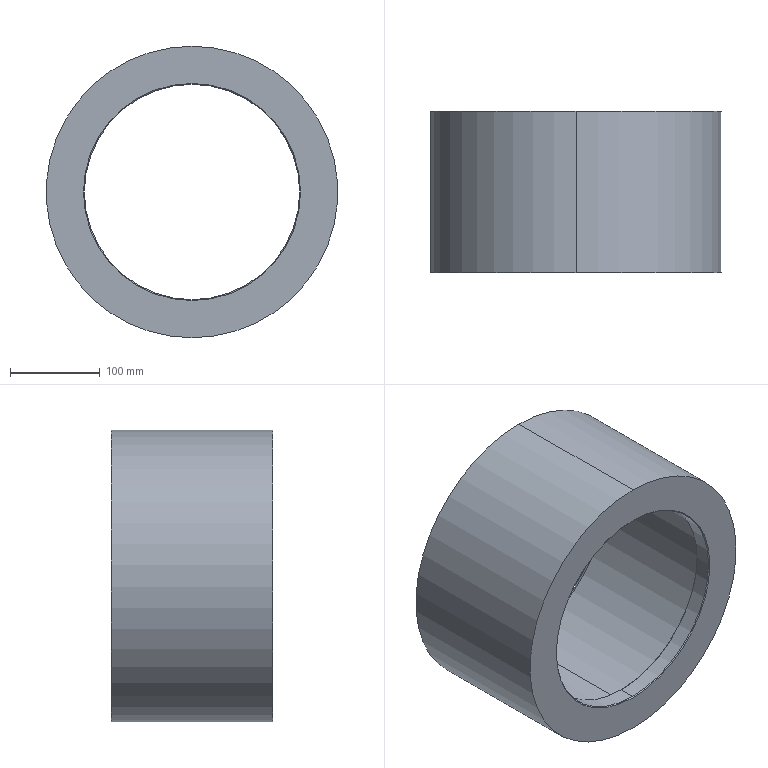Part | SolidWorks | features Chamfer 2, Extrusion 1, HoleWzd 1, ICE 1 | 1 solid | 31 faces | box 325 x 180 x 325 mm | volume 4860812 mm3 | cylinder 14 | cone 14 | plane 3 | commonest cylinder face diameters 6.8 x8 240 x2 270 x2 325 x2
STEP:
#1=CARTESIAN_POINT('',(148.,154.,-3.4));
#2=VERTEX_POINT('',#1);
#3=CARTESIAN_POINT('',(148.,154.,3.4));
#4=VERTEX_POINT('',#3);
#5=CARTESIAN_POINT('',(148.,154.,0.));
#6=DIRECTION('',(0.,1.,0.));
#7=DIRECTION('',(0.,0.,1.));
#8=AXIS2_PLACEMENT_3D('',#5,#6,#7);
#9=CIRCLE('',#8,3.4);
#10=EDGE_CURVE('',#2,#4,#9,.T.);
#11=ORIENTED_EDGE('',*,*,#10,.F.);
#12=CARTESIAN_POINT('',(148.,180.,-3.4));
#13=VERTEX_POINT('',#12);
#14=CARTESIAN_POINT('',(148.,180.,-3.4));
#15=DIRECTION('',(0.,1.,0.));
#16=VECTOR('',#15,1000.);
#17=LINE('',#14,#16);
#18=EDGE_CURVE('',#2,#13,#17,.T.);
#19=ORIENTED_EDGE('',*,*,#18,.T.);
#20=CARTESIAN_POINT('',(148.,180.,3.4));
#21=VERTEX_POINT('',#20);
#22=CARTESIAN_POINT('',(148.,180.,0.));
#23=DIRECTION('',(0.,1.,0.));
#24=DIRECTION('',(0.,0.,1.));
#25=AXIS2_PLACEMENT_3D('',#22,#23,#24);
#26=CIRCLE('',#25,3.4);
#27=EDGE_CURVE('',#13,#21,#26,.T.);
#28=ORIENTED_EDGE('',*,*,#27,.T.);
#29=CARTESIAN_POINT('',(148.,180.,3.4));
#30=DIRECTION('',(0.,1.,0.));
#31=VECTOR('',#30,1000.);
#32=LINE('',#29,#31);
#33=EDGE_CURVE('',#4,#21,#32,.T.);
#34=ORIENTED_EDGE('',*,*,#33,.F.);
#35=EDGE_LOOP('',(#11,#19,#28,#34));
#36=FACE_OUTER_BOUND('',#35,.T.);
#37=CARTESIAN_POINT('',(148.,180.,0.));
#38=DIRECTION('',(0.,1.,0.));
#39=DIRECTION('',(0.,0.,1.));
#40=AXIS2_PLACEMENT_3D('',#37,#38,#39);
#41=CYLINDRICAL_SURFACE('',#40,3.4);
#42=ADVANCED_FACE('',(#36),#41,.F.);
#43=CARTESIAN_POINT('',(148.,151.957,0.));
#44=VERTEX_POINT('',#43);
#45=CARTESIAN_POINT('',(148.,154.,3.4));
#46=DIRECTION('',(0.,0.515,0.8572));
#47=VECTOR('',#46,1000.);
#48=LINE('',#45,#47);
#49=EDGE_CURVE('',#44,#4,#48,.T.);
#50=ORIENTED_EDGE('',*,*,#49,.F.);
#51=CARTESIAN_POINT('',(148.,154.,-3.4));
#52=DIRECTION('',(0.,0.515,-0.8572));
#53=VECTOR('',#52,1000.);
#54=LINE('',#51,#53);
#55=EDGE_CURVE('',#44,#2,#54,.T.);
#56=ORIENTED_EDGE('',*,*,#55,.T.);
#57=ORIENTED_EDGE('',*,*,#10,.T.);
#58=EDGE_LOOP('',(#50,#56,#57));
#59=FACE_OUTER_BOUND('',#58,.T.);
#60=CARTESIAN_POINT('',(148.,154.,0.));
#61=DIRECTION('',(0.,1.,0.));
#62=DIRECTION('',(0.,0.,1.));
#63=AXIS2_PLACEMENT_3D('',#60,#61,#62);
#64=CONICAL_SURFACE('',#63,3.4,1.03);
#65=ADVANCED_FACE('',(#59),#64,.F.);
#66=CARTESIAN_POINT('',(0.,154.,144.6));
#67=VERTEX_POINT('',#66);
#68=CARTESIAN_POINT('',(0.,154.,151.4));
#69=VERTEX_POINT('',#68);
#70=CARTESIAN_POINT('',(0.,154.,148.));
#71=DIRECTION('',(0.,1.,0.));
#72=DIRECTION('',(0.,0.,1.));
#73=AXIS2_PLACEMENT_3D('',#70,#71,#72);
#74=CIRCLE('',#73,3.4);
#75=EDGE_CURVE('',#67,#69,#74,.T.);
#76=ORIENTED_EDGE('',*,*,#75,.F.);
#77=CARTESIAN_POINT('',(0.,180.,144.6));
#78=VERTEX_POINT('',#77);
#79=CARTESIAN_POINT('',(0.,180.,144.6));
#80=DIRECTION('',(0.,1.,0.));
#81=VECTOR('',#80,1000.);
#82=LINE('',#79,#81);
#83=EDGE_CURVE('',#67,#78,#82,.T.);
#84=ORIENTED_EDGE('',*,*,#83,.T.);
#85=CARTESIAN_POINT('',(0.,180.,151.4));
#86=VERTEX_POINT('',#85);
#87=CARTESIAN_POINT('',(0.,180.,148.));
#88=DIRECTION('',(0.,1.,0.));
#89=DIRECTION('',(0.,0.,1.));
#90=AXIS2_PLACEMENT_3D('',#87,#88,#89);
#91=CIRCLE('',#90,3.4);
#92=EDGE_CURVE('',#78,#86,#91,.T.);
#93=ORIENTED_EDGE('',*,*,#92,.T.);
#94=CARTESIAN_POINT('',(0.,180.,151.4));
#95=DIRECTION('',(0.,1.,0.));
#96=VECTOR('',#95,1000.);
#97=LINE('',#94,#96);
#98=EDGE_CURVE('',#69,#86,#97,.T.);
#99=ORIENTED_EDGE('',*,*,#98,.F.);
#100=EDGE_LOOP('',(#76,#84,#93,#99));
#101=FACE_OUTER_BOUND('',#100,.T.);
#102=CARTESIAN_POINT('',(0.,180.,148.));
#103=DIRECTION('',(0.,1.,0.));
#104=DIRECTION('',(0.,0.,1.));
#105=AXIS2_PLACEMENT_3D('',#102,#103,#104);
#106=CYLINDRICAL_SURFACE('',#105,3.4);
#107=ADVANCED_FACE('',(#101),#106,.F.);
#108=CARTESIAN_POINT('',(0.,151.957,148.));
#109=VERTEX_POINT('',#108);
#110=CARTESIAN_POINT('',(0.,154.,151.4));
#111=DIRECTION('',(0.,0.515,0.8572));
#112=VECTOR('',#111,1000.);
#113=LINE('',#110,#112);
#114=EDGE_CURVE('',#109,#69,#113,.T.);
#115=ORIENTED_EDGE('',*,*,#114,.F.);
#116=CARTESIAN_POINT('',(0.,154.,144.6));
#117=DIRECTION('',(0.,0.515,-0.8572));
#118=VECTOR('',#117,1000.);
#119=LINE('',#116,#118);
#120=EDGE_CURVE('',#109,#67,#119,.T.);
#121=ORIENTED_EDGE('',*,*,#120,.T.);
#122=ORIENTED_EDGE('',*,*,#75,.T.);
#123=EDGE_LOOP('',(#115,#121,#122));
#124=FACE_OUTER_BOUND('',#123,.T.);
#125=CARTESIAN_POINT('',(0.,154.,148.));
#126=DIRECTION('',(0.,1.,0.));
#127=DIRECTION('',(0.,0.,1.));
#128=AXIS2_PLACEMENT_3D('',#125,#126,#127);
#129=CONICAL_SURFACE('',#128,3.4,1.03);
#130=ADVANCED_FACE('',(#124),#129,.F.);
#131=CARTESIAN_POINT('',(-148.,154.,-3.4));
#132=VERTEX_POINT('',#131);
#133=CARTESIAN_POINT('',(-148.,154.,3.4));
#134=VERTEX_POINT('',#133);
#135=CARTESIAN_POINT('',(-148.,154.,0.));
#136=DIRECTION('',(0.,1.,0.));
#137=DIRECTION('',(0.,0.,1.));
#138=AXIS2_PLACEMENT_3D('',#135,#136,#137);
#139=CIRCLE('',#138,3.4);
#140=EDGE_CURVE('',#132,#134,#139,.T.);
#141=ORIENTED_EDGE('',*,*,#140,.F.);
#142=CARTESIAN_POINT('',(-148.,180.,-3.4));
#143=VERTEX_POINT('',#142);
#144=CARTESIAN_POINT('',(-148.,180.,-3.4));
#145=DIRECTION('',(0.,1.,0.));
#146=VECTOR('',#145,1000.);
#147=LINE('',#144,#146);
#148=EDGE_CURVE('',#132,#143,#147,.T.);
#149=ORIENTED_EDGE('',*,*,#148,.T.);
#150=CARTESIAN_POINT('',(-148.,180.,3.4));
#151=VERTEX_POINT('',#150);
#152=CARTESIAN_POINT('',(-148.,180.,0.));
#153=DIRECTION('',(0.,1.,0.));
#154=DIRECTION('',(0.,0.,1.));
#155=AXIS2_PLACEMENT_3D('',#152,#153,#154);
#156=CIRCLE('',#155,3.4);
#157=EDGE_CURVE('',#143,#151,#156,.T.);
#158=ORIENTED_EDGE('',*,*,#157,.T.);
#159=CARTESIAN_POINT('',(-148.,180.,3.4));
#160=DIRECTION('',(0.,1.,0.));
#161=VECTOR('',#160,1000.);
#162=LINE('',#159,#161);
#163=EDGE_CURVE('',#134,#151,#162,.T.);
#164=ORIENTED_EDGE('',*,*,#163,.F.);
#165=EDGE_LOOP('',(#141,#149,#158,#164));
#166=FACE_OUTER_BOUND('',#165,.T.);
#167=CARTESIAN_POINT('',(-148.,180.,0.));
#168=DIRECTION('',(0.,1.,0.));
#169=DIRECTION('',(0.,0.,1.));
#170=AXIS2_PLACEMENT_3D('',#167,#168,#169);
#171=CYLINDRICAL_SURFACE('',#170,3.4);
#172=ADVANCED_FACE('',(#166),#171,.F.);
#173=CARTESIAN_POINT('',(-148.,151.957,0.));
#174=VERTEX_POINT('',#173);
#175=CARTESIAN_POINT('',(-148.,154.,3.4));
#176=DIRECTION('',(0.,0.515,0.8572));
#177=VECTOR('',#176,1000.);
#178=LINE('',#175,#177);
#179=EDGE_CURVE('',#174,#134,#178,.T.);
#180=ORIENTED_EDGE('',*,*,#179,.F.);
#181=CARTESIAN_POINT('',(-148.,154.,-3.4));
#182=DIRECTION('',(0.,0.515,-0.8572));
#183=VECTOR('',#182,1000.);
#184=LINE('',#181,#183);
#185=EDGE_CURVE('',#174,#132,#184,.T.);
#186=ORIENTED_EDGE('',*,*,#185,.T.);
#187=ORIENTED_EDGE('',*,*,#140,.T.);
#188=EDGE_LOOP('',(#180,#186,#187));
#189=FACE_OUTER_BOUND('',#188,.T.);
#190=CARTESIAN_POINT('',(-148.,154.,0.));
#191=DIRECTION('',(0.,1.,0.));
#192=DIRECTION('',(0.,0.,1.));
#193=AXIS2_PLACEMENT_3D('',#190,#191,#192);
#194=CONICAL_SURFACE('',#193,3.4,1.03);
#195=ADVANCED_FACE('',(#189),#194,.F.);
#196=CARTESIAN_POINT('',(0.,154.,-151.4));
#197=VERTEX_POINT('',#196);
#198=CARTESIAN_POINT('',(0.,154.,-144.6));
#199=VERTEX_POINT('',#198);
#200=CARTESIAN_POINT('',(0.,154.,-148.));
#201=DIRECTION('',(0.,1.,0.));
#202=DIRECTION('',(0.,0.,1.));
#203=AXIS2_PLACEMENT_3D('',#200,#201,#202);
#204=CIRCLE('',#203,3.4);
#205=EDGE_CURVE('',#197,#199,#204,.T.);
#206=ORIENTED_EDGE('',*,*,#205,.F.);
#207=CARTESIAN_POINT('',(0.,180.,-151.4));
#208=VERTEX_POINT('',#207);
#209=CARTESIAN_POINT('',(0.,180.,-151.4));
#210=DIRECTION('',(0.,1.,0.));
#211=VECTOR('',#210,1000.);
#212=LINE('',#209,#211);
#213=EDGE_CURVE('',#197,#208,#212,.T.);
#214=ORIENTED_EDGE('',*,*,#213,.T.);
#215=CARTESIAN_POINT('',(0.,180.,-144.6));
#216=VERTEX_POINT('',#215);
#217=CARTESIAN_POINT('',(0.,180.,-148.));
#218=DIRECTION('',(0.,1.,0.));
#219=DIRECTION('',(0.,0.,1.));
#220=AXIS2_PLACEMENT_3D('',#217,#218,#219);
#221=CIRCLE('',#220,3.4);
#222=EDGE_CURVE('',#208,#216,#221,.T.);
#223=ORIENTED_EDGE('',*,*,#222,.T.);
#224=CARTESIAN_POINT('',(0.,180.,-144.6));
#225=DIRECTION('',(0.,1.,0.));
#226=VECTOR('',#225,1000.);
#227=LINE('',#224,#226);
#228=EDGE_CURVE('',#199,#216,#227,.T.);
#229=ORIENTED_EDGE('',*,*,#228,.F.);
#230=EDGE_LOOP('',(#206,#214,#223,#229));
#231=FACE_OUTER_BOUND('',#230,.T.);
#232=CARTESIAN_POINT('',(0.,180.,-148.));
#233=DIRECTION('',(0.,1.,0.));
#234=DIRECTION('',(0.,0.,1.));
#235=AXIS2_PLACEMENT_3D('',#232,#233,#234);
#236=CYLINDRICAL_SURFACE('',#235,3.4);
#237=ADVANCED_FACE('',(#231),#236,.F.);
#238=CARTESIAN_POINT('',(0.,151.957,-148.));
#239=VERTEX_POINT('',#238);
#240=CARTESIAN_POINT('',(0.,154.,-144.6));
#241=DIRECTION('',(0.,0.515,0.8572));
#242=VECTOR('',#241,1000.);
#243=LINE('',#240,#242);
#244=EDGE_CURVE('',#239,#199,#243,.T.);
#245=ORIENTED_EDGE('',*,*,#244,.F.);
#246=CARTESIAN_POINT('',(0.,154.,-151.4));
#247=DIRECTION('',(0.,0.515,-0.8572));
#248=VECTOR('',#247,1000.);
#249=LINE('',#246,#248);
#250=EDGE_CURVE('',#239,#197,#249,.T.);
#251=ORIENTED_EDGE('',*,*,#250,.T.);
#252=ORIENTED_EDGE('',*,*,#205,.T.);
#253=EDGE_LOOP('',(#245,#251,#252));
#254=FACE_OUTER_BOUND('',#253,.T.);
#255=CARTESIAN_POINT('',(0.,154.,-148.));
#256=DIRECTION('',(0.,1.,0.));
#257=DIRECTION('',(0.,0.,1.));
#258=AXIS2_PLACEMENT_3D('',#255,#256,#257);
#259=CONICAL_SURFACE('',#258,3.4,1.03);
#260=ADVANCED_FACE('',(#254),#259,.F.);
#261=CARTESIAN_POINT('',(0.,1.,120.));
#262=VERTEX_POINT('',#261);
#263=CARTESIAN_POINT('',(0.,1.,-120.));
#264=VERTEX_POINT('',#263);
#265=CARTESIAN_POINT('',(0.,1.,0.));
#266=DIRECTION('',(0.,-1.,0.));
#267=DIRECTION('',(0.,0.,1.));
#268=AXIS2_PLACEMENT_3D('',#265,#266,#267);
#269=CIRCLE('',#268,120.);
#270=EDGE_CURVE('',#262,#264,#269,.T.);
#271=ORIENTED_EDGE('',*,*,#270,.F.);
#272=CARTESIAN_POINT('',(0.,0.,121.));
#273=VERTEX_POINT('',#272);
#274=CARTESIAN_POINT('',(0.,0.,121.));
#275=DIRECTION('',(0.,-0.7071,0.7071));
#276=VECTOR('',#275,1000.);
#277=LINE('',#274,#276);
#278=EDGE_CURVE('',#262,#273,#277,.T.);
#279=ORIENTED_EDGE('',*,*,#278,.T.);
#280=CARTESIAN_POINT('',(0.,0.,-121.));
#281=VERTEX_POINT('',#280);
#282=CARTESIAN_POINT('',(0.,0.,0.));
#283=DIRECTION('',(0.,1.,0.));
#284=DIRECTION('',(0.,0.,1.));
#285=AXIS2_PLACEMENT_3D('',#282,#283,#284);
#286=CIRCLE('',#285,121.);
#287=EDGE_CURVE('',#281,#273,#286,.T.);
#288=ORIENTED_EDGE('',*,*,#287,.F.);
#289=CARTESIAN_POINT('',(0.,0.,-121.));
#290=DIRECTION('',(0.,-0.7071,-0.7071));
#291=VECTOR('',#290,1000.);
#292=LINE('',#289,#291);
#293=EDGE_CURVE('',#264,#281,#292,.T.);
#294=ORIENTED_EDGE('',*,*,#293,.F.);
#295=EDGE_LOOP('',(#271,#279,#288,#294));
#296=FACE_OUTER_BOUND('',#295,.T.);
#297=CARTESIAN_POINT('',(0.,0.,0.));
#298=DIRECTION('',(0.,-1.,0.));
#299=DIRECTION('',(0.,0.,-1.));
#300=AXIS2_PLACEMENT_3D('',#297,#298,#299);
#301=CONICAL_SURFACE('',#300,121.,0.7854);
#302=ADVANCED_FACE('',(#296),#301,.F.);
#303=CARTESIAN_POINT('',(0.,19.,-120.));
#304=VERTEX_POINT('',#303);
#305=CARTESIAN_POINT('',(0.,19.,120.));
#306=VERTEX_POINT('',#305);
#307=CARTESIAN_POINT('',(0.,19.,0.));
#308=DIRECTION('',(0.,1.,0.));
#309=DIRECTION('',(0.,0.,1.));
#310=AXIS2_PLACEMENT_3D('',#307,#308,#309);
#311=CIRCLE('',#310,120.);
#312=EDGE_CURVE('',#304,#306,#311,.T.);
#313=ORIENTED_EDGE('',*,*,#312,.F.);
#314=CARTESIAN_POINT('',(0.,20.,-121.));
#315=VERTEX_POINT('',#314);
#316=CARTESIAN_POINT('',(0.,19.,-120.));
#317=DIRECTION('',(0.,0.7071,-0.7071));
#318=VECTOR('',#317,1000.);
#319=LINE('',#316,#318);
#320=EDGE_CURVE('',#304,#315,#319,.T.);
#321=ORIENTED_EDGE('',*,*,#320,.T.);
#322=CARTESIAN_POINT('',(0.,20.,121.));
#323=VERTEX_POINT('',#322);
#324=CARTESIAN_POINT('',(0.,20.,0.));
#325=DIRECTION('',(0.,-1.,0.));
#326=DIRECTION('',(0.,0.,1.));
#327=AXIS2_PLACEMENT_3D('',#324,#325,#326);
#328=CIRCLE('',#327,121.);
#329=EDGE_CURVE('',#323,#315,#328,.T.);
#330=ORIENTED_EDGE('',*,*,#329,.F.);
#331=CARTESIAN_POINT('',(0.,19.,120.));
#332=DIRECTION('',(0.,0.7071,0.7071));
#333=VECTOR('',#332,1000.);
#334=LINE('',#331,#333);
#335=EDGE_CURVE('',#306,#323,#334,.T.);
#336=ORIENTED_EDGE('',*,*,#335,.F.);
#337=EDGE_LOOP('',(#313,#321,#330,#336));
#338=FACE_OUTER_BOUND('',#337,.T.);
#339=CARTESIAN_POINT('',(0.,19.,0.));
#340=DIRECTION('',(0.,1.,0.));
#341=DIRECTION('',(0.,0.,1.));
#342=AXIS2_PLACEMENT_3D('',#339,#340,#341);
#343=CONICAL_SURFACE('',#342,120.,0.7854);
#344=ADVANCED_FACE('',(#338),#343,.F.);
#345=CARTESIAN_POINT('',(0.,177.,-135.));
#346=VERTEX_POINT('',#345);
#347=CARTESIAN_POINT('',(0.,177.,135.));
#348=VERTEX_POINT('',#347);
#349=CARTESIAN_POINT('',(0.,177.,0.));
#350=DIRECTION('',(0.,1.,0.));
#351=DIRECTION('',(0.,0.,1.));
#352=AXIS2_PLACEMENT_3D('',#349,#350,#351);
#353=CIRCLE('',#352,135.);
#354=EDGE_CURVE('',#346,#348,#353,.T.);
#355=ORIENTED_EDGE('',*,*,#354,.F.);
#356=CARTESIAN_POINT('',(0.,180.,-136.));
#357=VERTEX_POINT('',#356);
#358=CARTESIAN_POINT('',(0.,177.,-135.));
#359=DIRECTION('',(0.,0.9487,-0.3162));
#360=VECTOR('',#359,1000.);
#361=LINE('',#358,#360);
#362=EDGE_CURVE('',#346,#357,#361,.T.);
#363=ORIENTED_EDGE('',*,*,#362,.T.);
#364=CARTESIAN_POINT('',(0.,180.,136.));
#365=VERTEX_POINT('',#364);
#366=CARTESIAN_POINT('',(0.,180.,0.));
#367=DIRECTION('',(0.,-1.,0.));
#368=DIRECTION('',(0.,0.,1.));
#369=AXIS2_PLACEMENT_3D('',#366,#367,#368);
#370=CIRCLE('',#369,136.);
#371=EDGE_CURVE('',#365,#357,#370,.T.);
#372=ORIENTED_EDGE('',*,*,#371,.F.);
#373=CARTESIAN_POINT('',(0.,177.,135.));
#374=DIRECTION('',(0.,0.9487,0.3162));
#375=VECTOR('',#374,1000.);
#376=LINE('',#373,#375);
#377=EDGE_CURVE('',#348,#365,#376,.T.);
#378=ORIENTED_EDGE('',*,*,#377,.F.);
#379=EDGE_LOOP('',(#355,#363,#372,#378));
#380=FACE_OUTER_BOUND('',#379,.T.);
#381=CARTESIAN_POINT('',(0.,177.,0.));
#382=DIRECTION('',(0.,1.,0.));
#383=DIRECTION('',(0.,0.,1.));
#384=AXIS2_PLACEMENT_3D('',#381,#382,#383);
#385=CONICAL_SURFACE('',#384,135.,0.3218);
#386=ADVANCED_FACE('',(#380),#385,.F.);
#387=CARTESIAN_POINT('',(0.,20.,-135.));
#388=VERTEX_POINT('',#387);
#389=CARTESIAN_POINT('',(0.,20.,135.));
#390=VERTEX_POINT('',#389);
#391=CARTESIAN_POINT('',(0.,20.,0.));
#392=DIRECTION('',(0.,1.,0.));
#393=DIRECTION('',(0.,0.,1.));
#394=AXIS2_PLACEMENT_3D('',#391,#392,#393);
#395=CIRCLE('',#394,135.);
#396=EDGE_CURVE('',#388,#390,#395,.T.);
#397=ORIENTED_EDGE('',*,*,#396,.F.);
#398=CARTESIAN_POINT('',(0.,20.,-135.));
#399=DIRECTION('',(0.,1.,0.));
#400=VECTOR('',#399,1000.);
#401=LINE('',#398,#400);
#402=EDGE_CURVE('',#388,#346,#401,.T.);
#403=ORIENTED_EDGE('',*,*,#402,.T.);
#404=ORIENTED_EDGE('',*,*,#354,.T.);
#405=CARTESIAN_POINT('',(0.,20.,135.));
#406=DIRECTION('',(0.,1.,0.));
#407=VECTOR('',#406,1000.);
#408=LINE('',#405,#407);
#409=EDGE_CURVE('',#390,#348,#408,.T.);
#410=ORIENTED_EDGE('',*,*,#409,.F.);
#411=EDGE_LOOP('',(#397,#403,#404,#410));
#412=FACE_OUTER_BOUND('',#411,.T.);
#413=CARTESIAN_POINT('',(0.,20.,0.));
#414=DIRECTION('',(0.,1.,0.));
#415=DIRECTION('',(0.,0.,1.));
#416=AXIS2_PLACEMENT_3D('',#413,#414,#415);
#417=CYLINDRICAL_SURFACE('',#416,135.);
#418=ADVANCED_FACE('',(#412),#417,.F.);
#419=CARTESIAN_POINT('',(0.,180.,162.5));
#420=VERTEX_POINT('',#419);
#421=CARTESIAN_POINT('',(0.,180.,-162.5));
#422=VERTEX_POINT('',#421);
#423=CARTESIAN_POINT('',(0.,180.,0.));
#424=DIRECTION('',(0.,1.,0.));
#425=DIRECTION('',(0.,0.,1.));
#426=AXIS2_PLACEMENT_3D('',#423,#424,#425);
#427=CIRCLE('',#426,162.5);
#428=EDGE_CURVE('',#420,#422,#427,.T.);
#429=ORIENTED_EDGE('',*,*,#428,.F.);
#430=CARTESIAN_POINT('',(0.,0.,162.5));
#431=VERTEX_POINT('',#430);
#432=CARTESIAN_POINT('',(0.,180.,162.5));
#433=DIRECTION('',(0.,-1.,0.));
#434=VECTOR('',#433,1000.);
#435=LINE('',#432,#434);
#436=EDGE_CURVE('',#420,#431,#435,.T.);
#437=ORIENTED_EDGE('',*,*,#436,.T.);
#438=CARTESIAN_POINT('',(0.,0.,-162.5));
#439=VERTEX_POINT('',#438);
#440=CARTESIAN_POINT('',(0.,0.,0.));
#441=DIRECTION('',(0.,1.,0.));
#442=DIRECTION('',(0.,0.,1.));
#443=AXIS2_PLACEMENT_3D('',#440,#441,#442);
#444=CIRCLE('',#443,162.5);
#445=EDGE_CURVE('',#431,#439,#444,.T.);
#446=ORIENTED_EDGE('',*,*,#445,.T.);
#447=CARTESIAN_POINT('',(0.,180.,-162.5));
#448=DIRECTION('',(0.,-1.,0.));
#449=VECTOR('',#448,1000.);
#450=LINE('',#447,#449);
#451=EDGE_CURVE('',#422,#439,#450,.T.);
#452=ORIENTED_EDGE('',*,*,#451,.F.);
#453=EDGE_LOOP('',(#429,#437,#446,#452));
#454=FACE_OUTER_BOUND('',#453,.T.);
#455=CARTESIAN_POINT('',(0.,180.,0.));
#456=DIRECTION('',(0.,-1.,0.));
#457=DIRECTION('',(0.,0.,-1.));
#458=AXIS2_PLACEMENT_3D('',#455,#456,#457);
#459=CYLINDRICAL_SURFACE('',#458,162.5);
#460=ADVANCED_FACE('',(#454),#459,.T.);
#461=ORIENTED_EDGE('',*,*,#312,.T.);
#462=CARTESIAN_POINT('',(0.,180.,120.));
#463=DIRECTION('',(0.,-1.,0.));
#464=VECTOR('',#463,1000.);
#465=LINE('',#462,#464);
#466=EDGE_CURVE('',#306,#262,#465,.T.);
#467=ORIENTED_EDGE('',*,*,#466,.T.);
#468=ORIENTED_EDGE('',*,*,#270,.T.);
#469=CARTESIAN_POINT('',(0.,180.,-120.));
#470=DIRECTION('',(0.,-1.,0.));
#471=VECTOR('',#470,1000.);
#472=LINE('',#469,#471);
#473=EDGE_CURVE('',#304,#264,#472,.T.);
#474=ORIENTED_EDGE('',*,*,#473,.F.);
#475=EDGE_LOOP('',(#461,#467,#468,#474));
#476=FACE_OUTER_BOUND('',#475,.T.);
#477=CARTESIAN_POINT('',(0.,180.,0.));
#478=DIRECTION('',(0.,-1.,0.));
#479=DIRECTION('',(0.,0.,-1.));
#480=AXIS2_PLACEMENT_3D('',#477,#478,#479);
#481=CYLINDRICAL_SURFACE('',#480,120.);
#482=ADVANCED_FACE('',(#476),#481,.F.);
#483=ORIENTED_EDGE('',*,*,#466,.F.);
#484=CARTESIAN_POINT('',(0.,19.,0.));
#485=DIRECTION('',(0.,1.,0.));
#486=DIRECTION('',(0.,0.,1.));
#487=AXIS2_PLACEMENT_3D('',#484,#485,#486);
#488=CIRCLE('',#487,120.);
#489=EDGE_CURVE('',#306,#304,#488,.T.);
#490=ORIENTED_EDGE('',*,*,#489,.T.);
#491=ORIENTED_EDGE('',*,*,#473,.T.);
#492=CARTESIAN_POINT('',(0.,1.,0.));
#493=DIRECTION('',(0.,-1.,0.));
#494=DIRECTION('',(0.,0.,1.));
#495=AXIS2_PLACEMENT_3D('',#492,#493,#494);
#496=CIRCLE('',#495,120.);
#497=EDGE_CURVE('',#264,#262,#496,.T.);
#498=ORIENTED_EDGE('',*,*,#497,.T.);
#499=EDGE_LOOP('',(#483,#490,#491,#498));
#500=FACE_OUTER_BOUND('',#499,.T.);
#501=CARTESIAN_POINT('',(0.,180.,0.));
#502=DIRECTION('',(0.,-1.,0.));
#503=DIRECTION('',(0.,0.,-1.));
#504=AXIS2_PLACEMENT_3D('',#501,#502,#503);
#505=CYLINDRICAL_SURFACE('',#504,120.);
#506=ADVANCED_FACE('',(#500),#505,.F.);
#507=CARTESIAN_POINT('',(148.,180.,0.));
#508=DIRECTION('',(0.,1.,0.));
#509=DIRECTION('',(0.,0.,1.));
#510=AXIS2_PLACEMENT_3D('',#507,#508,#509);
#511=CIRCLE('',#510,3.4);
#512=EDGE_CURVE('',#21,#13,#511,.T.);
#513=ORIENTED_EDGE('',*,*,#512,.F.);
#514=ORIENTED_EDGE('',*,*,#27,.F.);
#515=EDGE_LOOP('',(#513,#514));
#516=FACE_BOUND('',#515,.T.);
#517=CARTESIAN_POINT('',(0.,180.,148.));
#518=DIRECTION('',(0.,1.,0.));
#519=DIRECTION('',(0.,0.,1.));
#520=AXIS2_PLACEMENT_3D('',#517,#518,#519);
#521=CIRCLE('',#520,3.4);
#522=EDGE_CURVE('',#86,#78,#521,.T.);
#523=ORIENTED_EDGE('',*,*,#522,.F.);
#524=ORIENTED_EDGE('',*,*,#92,.F.);
#525=EDGE_LOOP('',(#523,#524));
#526=FACE_BOUND('',#525,.T.);
#527=CARTESIAN_POINT('',(-148.,180.,0.));
#528=DIRECTION('',(0.,1.,0.));
#529=DIRECTION('',(0.,0.,1.));
#530=AXIS2_PLACEMENT_3D('',#527,#528,#529);
#531=CIRCLE('',#530,3.4);
#532=EDGE_CURVE('',#151,#143,#531,.T.);
#533=ORIENTED_EDGE('',*,*,#532,.F.);
#534=ORIENTED_EDGE('',*,*,#157,.F.);
#535=EDGE_LOOP('',(#533,#534));
#536=FACE_BOUND('',#535,.T.);
#537=CARTESIAN_POINT('',(0.,180.,-148.));
#538=DIRECTION('',(0.,1.,0.));
#539=DIRECTION('',(0.,0.,1.));
#540=AXIS2_PLACEMENT_3D('',#537,#538,#539);
#541=CIRCLE('',#540,3.4);
#542=EDGE_CURVE('',#216,#208,#541,.T.);
#543=ORIENTED_EDGE('',*,*,#542,.F.);
#544=ORIENTED_EDGE('',*,*,#222,.F.);
#545=EDGE_LOOP('',(#543,#544));
#546=FACE_BOUND('',#545,.T.);
#547=ORIENTED_EDGE('',*,*,#371,.T.);
#548=CARTESIAN_POINT('',(0.,180.,0.));
#549=DIRECTION('',(0.,-1.,0.));
#550=DIRECTION('',(0.,0.,1.));
#551=AXIS2_PLACEMENT_3D('',#548,#549,#550);
#552=CIRCLE('',#551,136.);
#553=EDGE_CURVE('',#357,#365,#552,.T.);
#554=ORIENTED_EDGE('',*,*,#553,.T.);
#555=EDGE_LOOP('',(#547,#554));
#556=FACE_BOUND('',#555,.T.);
#557=CARTESIAN_POINT('',(0.,180.,0.));
#558=DIRECTION('',(0.,1.,0.));
#559=DIRECTION('',(0.,0.,1.));
#560=AXIS2_PLACEMENT_3D('',#557,#558,#559);
#561=CIRCLE('',#560,162.5);
#562=EDGE_CURVE('',#422,#420,#561,.T.);
#563=ORIENTED_EDGE('',*,*,#562,.T.);
#564=ORIENTED_EDGE('',*,*,#428,.T.);
#565=EDGE_LOOP('',(#563,#564));
#566=FACE_OUTER_BOUND('',#565,.T.);
#567=CARTESIAN_POINT('',(0.,180.,0.));
#568=DIRECTION('',(0.,1.,0.));
#569=DIRECTION('',(0.,0.,1.));
#570=AXIS2_PLACEMENT_3D('',#567,#568,#569);
#571=PLANE('',#570);
#572=ADVANCED_FACE('',(#516,#526,#536,#546,#556,#566),#571,.T.);
#573=ORIENTED_EDGE('',*,*,#287,.T.);
#574=CARTESIAN_POINT('',(0.,0.,0.));
#575=DIRECTION('',(0.,1.,0.));
#576=DIRECTION('',(0.,0.,1.));
#577=AXIS2_PLACEMENT_3D('',#574,#575,#576);
#578=CIRCLE('',#577,121.);
#579=EDGE_CURVE('',#273,#281,#578,.T.);
#580=ORIENTED_EDGE('',*,*,#579,.T.);
#581=EDGE_LOOP('',(#573,#580));
#582=FACE_BOUND('',#581,.T.);
#583=CARTESIAN_POINT('',(0.,0.,0.));
#584=DIRECTION('',(0.,1.,0.));
#585=DIRECTION('',(0.,0.,1.));
#586=AXIS2_PLACEMENT_3D('',#583,#584,#585);
#587=CIRCLE('',#586,162.5);
#588=EDGE_CURVE('',#439,#431,#587,.T.);
#589=ORIENTED_EDGE('',*,*,#588,.F.);
#590=ORIENTED_EDGE('',*,*,#445,.F.);
#591=EDGE_LOOP('',(#589,#590));
#592=FACE_OUTER_BOUND('',#591,.T.);
#593=CARTESIAN_POINT('',(0.,0.,0.));
#594=DIRECTION('',(0.,1.,0.));
#595=DIRECTION('',(0.,0.,1.));
#596=AXIS2_PLACEMENT_3D('',#593,#594,#595);
#597=PLANE('',#596);
#598=ADVANCED_FACE('',(#582,#592),#597,.F.);
#599=ORIENTED_EDGE('',*,*,#436,.F.);
#600=ORIENTED_EDGE('',*,*,#562,.F.);
#601=ORIENTED_EDGE('',*,*,#451,.T.);
#602=ORIENTED_EDGE('',*,*,#588,.T.);
#603=EDGE_LOOP('',(#599,#600,#601,#602));
#604=FACE_OUTER_BOUND('',#603,.T.);
#605=CARTESIAN_POINT('',(0.,180.,0.));
#606=DIRECTION('',(0.,-1.,0.));
#607=DIRECTION('',(0.,0.,-1.));
#608=AXIS2_PLACEMENT_3D('',#605,#606,#607);
#609=CYLINDRICAL_SURFACE('',#608,162.5);
#610=ADVANCED_FACE('',(#604),#609,.T.);
#611=ORIENTED_EDGE('',*,*,#402,.F.);
#612=CARTESIAN_POINT('',(0.,20.,0.));
#613=DIRECTION('',(0.,1.,0.));
#614=DIRECTION('',(0.,0.,1.));
#615=AXIS2_PLACEMENT_3D('',#612,#613,#614);
#616=CIRCLE('',#615,135.);
#617=EDGE_CURVE('',#390,#388,#616,.T.);
#618=ORIENTED_EDGE('',*,*,#617,.F.);
#619=ORIENTED_EDGE('',*,*,#409,.T.);
#620=CARTESIAN_POINT('',(0.,177.,0.));
#621=DIRECTION('',(0.,1.,0.));
#622=DIRECTION('',(0.,0.,1.));
#623=AXIS2_PLACEMENT_3D('',#620,#621,#622);
#624=CIRCLE('',#623,135.);
#625=EDGE_CURVE('',#348,#346,#624,.T.);
#626=ORIENTED_EDGE('',*,*,#625,.T.);
#627=EDGE_LOOP('',(#611,#618,#619,#626));
#628=FACE_OUTER_BOUND('',#627,.T.);
#629=CARTESIAN_POINT('',(0.,20.,0.));
#630=DIRECTION('',(0.,1.,0.));
#631=DIRECTION('',(0.,0.,1.));
#632=AXIS2_PLACEMENT_3D('',#629,#630,#631);
#633=CYLINDRICAL_SURFACE('',#632,135.);
#634=ADVANCED_FACE('',(#628),#633,.F.);
#635=ORIENTED_EDGE('',*,*,#329,.T.);
#636=CARTESIAN_POINT('',(0.,20.,0.));
#637=DIRECTION('',(0.,-1.,0.));
#638=DIRECTION('',(0.,0.,1.));
#639=AXIS2_PLACEMENT_3D('',#636,#637,#638);
#640=CIRCLE('',#639,121.);
#641=EDGE_CURVE('',#315,#323,#640,.T.);
#642=ORIENTED_EDGE('',*,*,#641,.T.);
#643=EDGE_LOOP('',(#635,#642));
#644=FACE_BOUND('',#643,.T.);
#645=ORIENTED_EDGE('',*,*,#617,.T.);
#646=ORIENTED_EDGE('',*,*,#396,.T.);
#647=EDGE_LOOP('',(#645,#646));
#648=FACE_OUTER_BOUND('',#647,.T.);
#649=CARTESIAN_POINT('',(0.,20.,0.));
#650=DIRECTION('',(0.,1.,0.));
#651=DIRECTION('',(0.,0.,1.));
#652=AXIS2_PLACEMENT_3D('',#649,#650,#651);
#653=PLANE('',#652);
#654=ADVANCED_FACE('',(#644,#648),#653,.T.);
#655=ORIENTED_EDGE('',*,*,#362,.F.);
#656=ORIENTED_EDGE('',*,*,#625,.F.);
#657=ORIENTED_EDGE('',*,*,#377,.T.);
#658=ORIENTED_EDGE('',*,*,#553,.F.);
#659=EDGE_LOOP('',(#655,#656,#657,#658));
#660=FACE_OUTER_BOUND('',#659,.T.);
#661=CARTESIAN_POINT('',(0.,177.,0.));
#662=DIRECTION('',(0.,1.,0.));
#663=DIRECTION('',(0.,0.,1.));
#664=AXIS2_PLACEMENT_3D('',#661,#662,#663);
#665=CONICAL_SURFACE('',#664,135.,0.3218);
#666=ADVANCED_FACE('',(#660),#665,.F.);
#667=ORIENTED_EDGE('',*,*,#320,.F.);
#668=ORIENTED_EDGE('',*,*,#489,.F.);
#669=ORIENTED_EDGE('',*,*,#335,.T.);
#670=ORIENTED_EDGE('',*,*,#641,.F.);
#671=EDGE_LOOP('',(#667,#668,#669,#670));
#672=FACE_OUTER_BOUND('',#671,.T.);
#673=CARTESIAN_POINT('',(0.,19.,0.));
#674=DIRECTION('',(0.,1.,0.));
#675=DIRECTION('',(0.,0.,1.));
#676=AXIS2_PLACEMENT_3D('',#673,#674,#675);
#677=CONICAL_SURFACE('',#676,120.,0.7854);
#678=ADVANCED_FACE('',(#672),#677,.F.);
#679=ORIENTED_EDGE('',*,*,#278,.F.);
#680=ORIENTED_EDGE('',*,*,#497,.F.);
#681=ORIENTED_EDGE('',*,*,#293,.T.);
#682=ORIENTED_EDGE('',*,*,#579,.F.);
#683=EDGE_LOOP('',(#679,#680,#681,#682));
#684=FACE_OUTER_BOUND('',#683,.T.);
#685=CARTESIAN_POINT('',(0.,0.,0.));
#686=DIRECTION('',(0.,-1.,0.));
#687=DIRECTION('',(0.,0.,-1.));
#688=AXIS2_PLACEMENT_3D('',#685,#686,#687);
#689=CONICAL_SURFACE('',#688,121.,0.7854);
#690=ADVANCED_FACE('',(#684),#689,.F.);
#691=ORIENTED_EDGE('',*,*,#250,.F.);
#692=ORIENTED_EDGE('',*,*,#244,.T.);
#693=CARTESIAN_POINT('',(0.,154.,-148.));
#694=DIRECTION('',(0.,1.,0.));
#695=DIRECTION('',(0.,0.,1.));
#696=AXIS2_PLACEMENT_3D('',#693,#694,#695);
#697=CIRCLE('',#696,3.4);
#698=EDGE_CURVE('',#199,#197,#697,.T.);
#699=ORIENTED_EDGE('',*,*,#698,.T.);
#700=EDGE_LOOP('',(#691,#692,#699));
#701=FACE_OUTER_BOUND('',#700,.T.);
#702=CARTESIAN_POINT('',(0.,154.,-148.));
#703=DIRECTION('',(0.,1.,0.));
#704=DIRECTION('',(0.,0.,1.));
#705=AXIS2_PLACEMENT_3D('',#702,#703,#704);
#706=CONICAL_SURFACE('',#705,3.4,1.03);
#707=ADVANCED_FACE('',(#701),#706,.F.);
#708=ORIENTED_EDGE('',*,*,#213,.F.);
#709=ORIENTED_EDGE('',*,*,#698,.F.);
#710=ORIENTED_EDGE('',*,*,#228,.T.);
#711=ORIENTED_EDGE('',*,*,#542,.T.);
#712=EDGE_LOOP('',(#708,#709,#710,#711));
#713=FACE_OUTER_BOUND('',#712,.T.);
#714=CARTESIAN_POINT('',(0.,180.,-148.));
#715=DIRECTION('',(0.,1.,0.));
#716=DIRECTION('',(0.,0.,1.));
#717=AXIS2_PLACEMENT_3D('',#714,#715,#716);
#718=CYLINDRICAL_SURFACE('',#717,3.4);
#719=ADVANCED_FACE('',(#713),#718,.F.);
#720=ORIENTED_EDGE('',*,*,#185,.F.);
#721=ORIENTED_EDGE('',*,*,#179,.T.);
#722=CARTESIAN_POINT('',(-148.,154.,0.));
#723=DIRECTION('',(0.,1.,0.));
#724=DIRECTION('',(0.,0.,1.));
#725=AXIS2_PLACEMENT_3D('',#722,#723,#724);
#726=CIRCLE('',#725,3.4);
#727=EDGE_CURVE('',#134,#132,#726,.T.);
#728=ORIENTED_EDGE('',*,*,#727,.T.);
#729=EDGE_LOOP('',(#720,#721,#728));
#730=FACE_OUTER_BOUND('',#729,.T.);
#731=CARTESIAN_POINT('',(-148.,154.,0.));
#732=DIRECTION('',(0.,1.,0.));
#733=DIRECTION('',(0.,0.,1.));
#734=AXIS2_PLACEMENT_3D('',#731,#732,#733);
#735=CONICAL_SURFACE('',#734,3.4,1.03);
#736=ADVANCED_FACE('',(#730),#735,.F.);
#737=ORIENTED_EDGE('',*,*,#148,.F.);
#738=ORIENTED_EDGE('',*,*,#727,.F.);
#739=ORIENTED_EDGE('',*,*,#163,.T.);
#740=ORIENTED_EDGE('',*,*,#532,.T.);
#741=EDGE_LOOP('',(#737,#738,#739,#740));
#742=FACE_OUTER_BOUND('',#741,.T.);
#743=CARTESIAN_POINT('',(-148.,180.,0.));
#744=DIRECTION('',(0.,1.,0.));
#745=DIRECTION('',(0.,0.,1.));
#746=AXIS2_PLACEMENT_3D('',#743,#744,#745);
#747=CYLINDRICAL_SURFACE('',#746,3.4);
#748=ADVANCED_FACE('',(#742),#747,.F.);
#749=ORIENTED_EDGE('',*,*,#120,.F.);
#750=ORIENTED_EDGE('',*,*,#114,.T.);
#751=CARTESIAN_POINT('',(0.,154.,148.));
#752=DIRECTION('',(0.,1.,0.));
#753=DIRECTION('',(0.,0.,1.));
#754=AXIS2_PLACEMENT_3D('',#751,#752,#753);
#755=CIRCLE('',#754,3.4);
#756=EDGE_CURVE('',#69,#67,#755,.T.);
#757=ORIENTED_EDGE('',*,*,#756,.T.);
#758=EDGE_LOOP('',(#749,#750,#757));
#759=FACE_OUTER_BOUND('',#758,.T.);
#760=CARTESIAN_POINT('',(0.,154.,148.));
#761=DIRECTION('',(0.,1.,0.));
#762=DIRECTION('',(0.,0.,1.));
#763=AXIS2_PLACEMENT_3D('',#760,#761,#762);
#764=CONICAL_SURFACE('',#763,3.4,1.03);
#765=ADVANCED_FACE('',(#759),#764,.F.);
#766=ORIENTED_EDGE('',*,*,#83,.F.);
#767=ORIENTED_EDGE('',*,*,#756,.F.);
#768=ORIENTED_EDGE('',*,*,#98,.T.);
#769=ORIENTED_EDGE('',*,*,#522,.T.);
#770=EDGE_LOOP('',(#766,#767,#768,#769));
#771=FACE_OUTER_BOUND('',#770,.T.);
#772=CARTESIAN_POINT('',(0.,180.,148.));
#773=DIRECTION('',(0.,1.,0.));
#774=DIRECTION('',(0.,0.,1.));
#775=AXIS2_PLACEMENT_3D('',#772,#773,#774);
#776=CYLINDRICAL_SURFACE('',#775,3.4);
#777=ADVANCED_FACE('',(#771),#776,.F.);
#778=ORIENTED_EDGE('',*,*,#55,.F.);
#779=ORIENTED_EDGE('',*,*,#49,.T.);
#780=CARTESIAN_POINT('',(148.,154.,0.));
#781=DIRECTION('',(0.,1.,0.));
#782=DIRECTION('',(0.,0.,1.));
#783=AXIS2_PLACEMENT_3D('',#780,#781,#782);
#784=CIRCLE('',#783,3.4);
#785=EDGE_CURVE('',#4,#2,#784,.T.);
#786=ORIENTED_EDGE('',*,*,#785,.T.);
#787=EDGE_LOOP('',(#778,#779,#786));
#788=FACE_OUTER_BOUND('',#787,.T.);
#789=CARTESIAN_POINT('',(148.,154.,0.));
#790=DIRECTION('',(0.,1.,0.));
#791=DIRECTION('',(0.,0.,1.));
#792=AXIS2_PLACEMENT_3D('',#789,#790,#791);
#793=CONICAL_SURFACE('',#792,3.4,1.03);
#794=ADVANCED_FACE('',(#788),#793,.F.);
#795=ORIENTED_EDGE('',*,*,#18,.F.);
#796=ORIENTED_EDGE('',*,*,#785,.F.);
#797=ORIENTED_EDGE('',*,*,#33,.T.);
#798=ORIENTED_EDGE('',*,*,#512,.T.);
#799=EDGE_LOOP('',(#795,#796,#797,#798));
#800=FACE_OUTER_BOUND('',#799,.T.);
#801=CARTESIAN_POINT('',(148.,180.,0.));
#802=DIRECTION('',(0.,1.,0.));
#803=DIRECTION('',(0.,0.,1.));
#804=AXIS2_PLACEMENT_3D('',#801,#802,#803);
#805=CYLINDRICAL_SURFACE('',#804,3.4);
#806=ADVANCED_FACE('',(#800),#805,.F.);
#807=CLOSED_SHELL('',(#42,#65,#107,#130,#172,#195,#237,#260,#302,#344,#386,#418,#460,#482,#506,#572,#598,#610,#634,#654,#666,#678,#690,#707,#719,#736,#748,#765,#777,#794,#806));
#808=MANIFOLD_SOLID_BREP('',#807);
#809=CARTESIAN_POINT('',(0.,0.,0.));
#810=DIRECTION('',(0.,0.,1.));
#811=DIRECTION('',(1.,0.,0.));
#812=AXIS2_PLACEMENT_3D('',#809,#810,#811);
#813=(LENGTH_UNIT()NAMED_UNIT(*)SI_UNIT(.MILLI.,.METRE.));
#814=UNCERTAINTY_MEASURE_WITH_UNIT(LENGTH_MEASURE(0.00001),#813,'','');
#815=(NAMED_UNIT(*)PLANE_ANGLE_UNIT()SI_UNIT($,.RADIAN.));
#816=(NAMED_UNIT(*)SI_UNIT($,.STERADIAN.)SOLID_ANGLE_UNIT());
#817=(GEOMETRIC_REPRESENTATION_CONTEXT(3)GLOBAL_UNCERTAINTY_ASSIGNED_CONTEXT((#814))GLOBAL_UNIT_ASSIGNED_CONTEXT((#813,#815,#816))REPRESENTATION_CONTEXT('',''));
#818=ADVANCED_BREP_SHAPE_REPRESENTATION('',(#808,#812),#817);